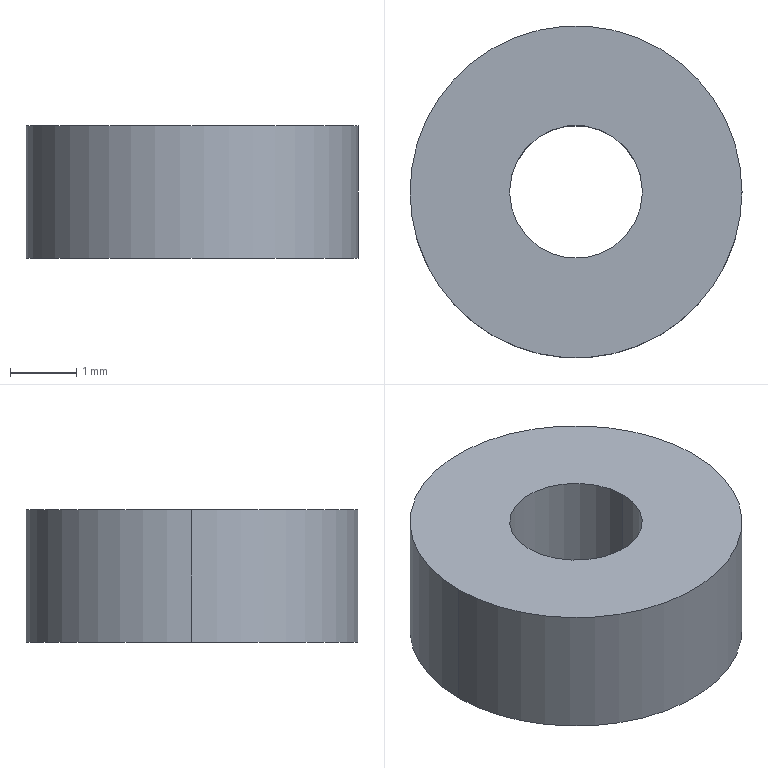Part | SolidWorks | features Extrusion 1 | 1 solid | 6 faces | box 5 x 5 x 2 mm | volume 32.987 mm3 | cylinder 4 | plane 2 | commonest cylinder face diameters 2 x2 5 x2
STEP:
#1=CARTESIAN_POINT('',(-221.5,0.,2.));
#2=VERTEX_POINT('',#1);
#3=CARTESIAN_POINT('',(-219.5,0.,2.));
#4=VERTEX_POINT('',#3);
#5=CARTESIAN_POINT('',(-220.5,0.,2.));
#6=DIRECTION('',(0.,0.,1.));
#7=DIRECTION('',(1.,0.,0.));
#8=AXIS2_PLACEMENT_3D('',#5,#6,#7);
#9=CIRCLE('',#8,1.);
#10=EDGE_CURVE('',#2,#4,#9,.T.);
#11=ORIENTED_EDGE('',*,*,#10,.T.);
#12=CARTESIAN_POINT('',(-219.5,0.,0.));
#13=VERTEX_POINT('',#12);
#14=CARTESIAN_POINT('',(-219.5,0.,2.));
#15=DIRECTION('',(0.,0.,-1.));
#16=VECTOR('',#15,1000.);
#17=LINE('',#14,#16);
#18=EDGE_CURVE('',#4,#13,#17,.T.);
#19=ORIENTED_EDGE('',*,*,#18,.T.);
#20=CARTESIAN_POINT('',(-221.5,0.,0.));
#21=VERTEX_POINT('',#20);
#22=CARTESIAN_POINT('',(-220.5,0.,0.));
#23=DIRECTION('',(0.,0.,1.));
#24=DIRECTION('',(1.,0.,0.));
#25=AXIS2_PLACEMENT_3D('',#22,#23,#24);
#26=CIRCLE('',#25,1.);
#27=EDGE_CURVE('',#21,#13,#26,.T.);
#28=ORIENTED_EDGE('',*,*,#27,.F.);
#29=CARTESIAN_POINT('',(-221.5,0.,2.));
#30=DIRECTION('',(0.,0.,-1.));
#31=VECTOR('',#30,1000.);
#32=LINE('',#29,#31);
#33=EDGE_CURVE('',#2,#21,#32,.T.);
#34=ORIENTED_EDGE('',*,*,#33,.F.);
#35=EDGE_LOOP('',(#11,#19,#28,#34));
#36=FACE_OUTER_BOUND('',#35,.T.);
#37=CARTESIAN_POINT('',(-220.5,0.,2.));
#38=DIRECTION('',(0.,0.,-1.));
#39=DIRECTION('',(-1.,0.,0.));
#40=AXIS2_PLACEMENT_3D('',#37,#38,#39);
#41=CYLINDRICAL_SURFACE('',#40,1.);
#42=ADVANCED_FACE('',(#36),#41,.F.);
#43=CARTESIAN_POINT('',(-218.,0.,2.));
#44=VERTEX_POINT('',#43);
#45=CARTESIAN_POINT('',(-223.,0.,2.));
#46=VERTEX_POINT('',#45);
#47=CARTESIAN_POINT('',(-220.5,0.,2.));
#48=DIRECTION('',(0.,0.,1.));
#49=DIRECTION('',(1.,0.,0.));
#50=AXIS2_PLACEMENT_3D('',#47,#48,#49);
#51=CIRCLE('',#50,2.5);
#52=EDGE_CURVE('',#44,#46,#51,.T.);
#53=ORIENTED_EDGE('',*,*,#52,.F.);
#54=CARTESIAN_POINT('',(-218.,0.,0.));
#55=VERTEX_POINT('',#54);
#56=CARTESIAN_POINT('',(-218.,0.,2.));
#57=DIRECTION('',(0.,0.,-1.));
#58=VECTOR('',#57,1000.);
#59=LINE('',#56,#58);
#60=EDGE_CURVE('',#44,#55,#59,.T.);
#61=ORIENTED_EDGE('',*,*,#60,.T.);
#62=CARTESIAN_POINT('',(-223.,0.,0.));
#63=VERTEX_POINT('',#62);
#64=CARTESIAN_POINT('',(-220.5,0.,0.));
#65=DIRECTION('',(0.,0.,1.));
#66=DIRECTION('',(1.,0.,0.));
#67=AXIS2_PLACEMENT_3D('',#64,#65,#66);
#68=CIRCLE('',#67,2.5);
#69=EDGE_CURVE('',#55,#63,#68,.T.);
#70=ORIENTED_EDGE('',*,*,#69,.T.);
#71=CARTESIAN_POINT('',(-223.,0.,2.));
#72=DIRECTION('',(0.,0.,-1.));
#73=VECTOR('',#72,1000.);
#74=LINE('',#71,#73);
#75=EDGE_CURVE('',#46,#63,#74,.T.);
#76=ORIENTED_EDGE('',*,*,#75,.F.);
#77=EDGE_LOOP('',(#53,#61,#70,#76));
#78=FACE_OUTER_BOUND('',#77,.T.);
#79=CARTESIAN_POINT('',(-220.5,0.,2.));
#80=DIRECTION('',(0.,0.,-1.));
#81=DIRECTION('',(-1.,0.,0.));
#82=AXIS2_PLACEMENT_3D('',#79,#80,#81);
#83=CYLINDRICAL_SURFACE('',#82,2.5);
#84=ADVANCED_FACE('',(#78),#83,.T.);
#85=CARTESIAN_POINT('',(-220.5,0.,2.));
#86=DIRECTION('',(0.,0.,1.));
#87=DIRECTION('',(1.,0.,0.));
#88=AXIS2_PLACEMENT_3D('',#85,#86,#87);
#89=CIRCLE('',#88,2.5);
#90=EDGE_CURVE('',#46,#44,#89,.T.);
#91=ORIENTED_EDGE('',*,*,#90,.T.);
#92=ORIENTED_EDGE('',*,*,#52,.T.);
#93=EDGE_LOOP('',(#91,#92));
#94=FACE_OUTER_BOUND('',#93,.T.);
#95=ORIENTED_EDGE('',*,*,#10,.F.);
#96=CARTESIAN_POINT('',(-220.5,0.,2.));
#97=DIRECTION('',(0.,0.,1.));
#98=DIRECTION('',(1.,0.,0.));
#99=AXIS2_PLACEMENT_3D('',#96,#97,#98);
#100=CIRCLE('',#99,1.);
#101=EDGE_CURVE('',#4,#2,#100,.T.);
#102=ORIENTED_EDGE('',*,*,#101,.F.);
#103=EDGE_LOOP('',(#95,#102));
#104=FACE_BOUND('',#103,.T.);
#105=CARTESIAN_POINT('',(-220.5,0.,2.));
#106=DIRECTION('',(0.,0.,1.));
#107=DIRECTION('',(1.,0.,0.));
#108=AXIS2_PLACEMENT_3D('',#105,#106,#107);
#109=PLANE('',#108);
#110=ADVANCED_FACE('',(#94,#104),#109,.T.);
#111=CARTESIAN_POINT('',(-220.5,0.,0.));
#112=DIRECTION('',(0.,0.,1.));
#113=DIRECTION('',(1.,0.,0.));
#114=AXIS2_PLACEMENT_3D('',#111,#112,#113);
#115=CIRCLE('',#114,2.5);
#116=EDGE_CURVE('',#63,#55,#115,.T.);
#117=ORIENTED_EDGE('',*,*,#116,.F.);
#118=ORIENTED_EDGE('',*,*,#69,.F.);
#119=EDGE_LOOP('',(#117,#118));
#120=FACE_OUTER_BOUND('',#119,.T.);
#121=ORIENTED_EDGE('',*,*,#27,.T.);
#122=CARTESIAN_POINT('',(-220.5,0.,0.));
#123=DIRECTION('',(0.,0.,1.));
#124=DIRECTION('',(1.,0.,0.));
#125=AXIS2_PLACEMENT_3D('',#122,#123,#124);
#126=CIRCLE('',#125,1.);
#127=EDGE_CURVE('',#13,#21,#126,.T.);
#128=ORIENTED_EDGE('',*,*,#127,.T.);
#129=EDGE_LOOP('',(#121,#128));
#130=FACE_BOUND('',#129,.T.);
#131=CARTESIAN_POINT('',(-220.5,0.,0.));
#132=DIRECTION('',(0.,0.,1.));
#133=DIRECTION('',(1.,0.,0.));
#134=AXIS2_PLACEMENT_3D('',#131,#132,#133);
#135=PLANE('',#134);
#136=ADVANCED_FACE('',(#120,#130),#135,.F.);
#137=ORIENTED_EDGE('',*,*,#60,.F.);
#138=ORIENTED_EDGE('',*,*,#90,.F.);
#139=ORIENTED_EDGE('',*,*,#75,.T.);
#140=ORIENTED_EDGE('',*,*,#116,.T.);
#141=EDGE_LOOP('',(#137,#138,#139,#140));
#142=FACE_OUTER_BOUND('',#141,.T.);
#143=CARTESIAN_POINT('',(-220.5,0.,2.));
#144=DIRECTION('',(0.,0.,-1.));
#145=DIRECTION('',(-1.,0.,0.));
#146=AXIS2_PLACEMENT_3D('',#143,#144,#145);
#147=CYLINDRICAL_SURFACE('',#146,2.5);
#148=ADVANCED_FACE('',(#142),#147,.T.);
#149=ORIENTED_EDGE('',*,*,#18,.F.);
#150=ORIENTED_EDGE('',*,*,#101,.T.);
#151=ORIENTED_EDGE('',*,*,#33,.T.);
#152=ORIENTED_EDGE('',*,*,#127,.F.);
#153=EDGE_LOOP('',(#149,#150,#151,#152));
#154=FACE_OUTER_BOUND('',#153,.T.);
#155=CARTESIAN_POINT('',(-220.5,0.,2.));
#156=DIRECTION('',(0.,0.,-1.));
#157=DIRECTION('',(-1.,0.,0.));
#158=AXIS2_PLACEMENT_3D('',#155,#156,#157);
#159=CYLINDRICAL_SURFACE('',#158,1.);
#160=ADVANCED_FACE('',(#154),#159,.F.);
#161=CLOSED_SHELL('',(#42,#84,#110,#136,#148,#160));
#162=MANIFOLD_SOLID_BREP('',#161);
#163=CARTESIAN_POINT('',(0.,0.,0.));
#164=DIRECTION('',(0.,0.,1.));
#165=DIRECTION('',(1.,0.,0.));
#166=AXIS2_PLACEMENT_3D('',#163,#164,#165);
#167=(LENGTH_UNIT()NAMED_UNIT(*)SI_UNIT(.MILLI.,.METRE.));
#168=UNCERTAINTY_MEASURE_WITH_UNIT(LENGTH_MEASURE(0.00001),#167,'','');
#169=(NAMED_UNIT(*)PLANE_ANGLE_UNIT()SI_UNIT($,.RADIAN.));
#170=(NAMED_UNIT(*)SI_UNIT($,.STERADIAN.)SOLID_ANGLE_UNIT());
#171=(GEOMETRIC_REPRESENTATION_CONTEXT(3)GLOBAL_UNCERTAINTY_ASSIGNED_CONTEXT((#168))GLOBAL_UNIT_ASSIGNED_CONTEXT((#167,#169,#170))REPRESENTATION_CONTEXT('',''));
#172=ADVANCED_BREP_SHAPE_REPRESENTATION('',(#162,#166),#171);